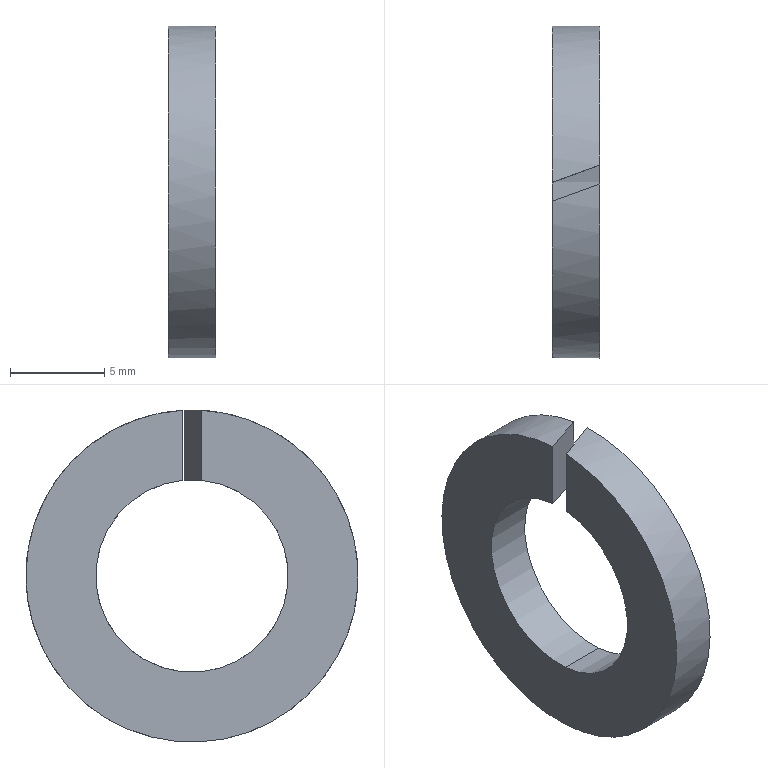Part | STEP file | KS B 1324 - No. 2 - 10 | 1 solid | 8 faces | box 2.5 x 17.6 x 17.6 mm | volume 394.643 mm3 | cylinder 4 | plane 4 | commonest cylinder face diameters 10.2 x2 17.6 x2
STEP:
#1=CARTESIAN_POINT('',(0.,0.,0.));
#2=DIRECTION('',(0.,0.,1.));
#3=DIRECTION('',(1.,0.,0.));
#4=AXIS2_PLACEMENT_3D('',#1,#2,#3);
#5=CARTESIAN_POINT('',(2.5,1.41,4.901));
#6=VERTEX_POINT('',#5);
#7=CARTESIAN_POINT('',(0.,0.5,5.075));
#8=VERTEX_POINT('',#7);
#9=CARTESIAN_POINT('',(2.5,1.41,4.901));
#10=CARTESIAN_POINT('',(1.682,1.112,4.987));
#11=CARTESIAN_POINT('',(0.8467,0.8082,5.045));
#12=CARTESIAN_POINT('',(0.,0.5,5.075));
#13=(BOUNDED_CURVE()B_SPLINE_CURVE(3,(#9,#10,#11,#12),.UNSPECIFIED.,.F.,.F.)B_SPLINE_CURVE_WITH_KNOTS((4,4),(4.432,4.614),.PIECEWISE_BEZIER_KNOTS.)CURVE()GEOMETRIC_REPRESENTATION_ITEM()RATIONAL_B_SPLINE_CURVE((1.,0.9972,0.9972,1.))REPRESENTATION_ITEM(''));
#14=CARTESIAN_POINT('',(0.,0.,0.));
#15=DIRECTION('',(1.,0.,0.));
#16=DIRECTION('',(0.,-0.08921,-0.996));
#17=AXIS2_PLACEMENT_3D('',#14,#15,#16);
#18=CYLINDRICAL_SURFACE('',#17,5.1);
#19=CARTESIAN_POINT('',(2.951,2.5));
#20=CARTESIAN_POINT('',(2.954,2.463));
#21=CARTESIAN_POINT('',(2.959,2.389));
#22=CARTESIAN_POINT('',(2.967,2.277));
#23=CARTESIAN_POINT('',(2.976,2.165));
#24=CARTESIAN_POINT('',(2.984,2.053));
#25=CARTESIAN_POINT('',(2.992,1.94));
#26=CARTESIAN_POINT('',(3.,1.828));
#27=CARTESIAN_POINT('',(3.009,1.715));
#28=CARTESIAN_POINT('',(3.017,1.602));
#29=CARTESIAN_POINT('',(3.025,1.488));
#30=CARTESIAN_POINT('',(3.033,1.375));
#31=CARTESIAN_POINT('',(3.042,1.261));
#32=CARTESIAN_POINT('',(3.05,1.147));
#33=CARTESIAN_POINT('',(3.058,1.033));
#34=CARTESIAN_POINT('',(3.067,0.9185));
#35=CARTESIAN_POINT('',(3.075,0.8041));
#36=CARTESIAN_POINT('',(3.083,0.6895));
#37=CARTESIAN_POINT('',(3.091,0.5749));
#38=CARTESIAN_POINT('',(3.1,0.4601));
#39=CARTESIAN_POINT('',(3.108,0.3452));
#40=CARTESIAN_POINT('',(3.116,0.2302));
#41=CARTESIAN_POINT('',(3.124,0.1151));
#42=CARTESIAN_POINT('',(3.13,0.03838));
#43=CARTESIAN_POINT('',(3.133,0.));
#44=B_SPLINE_CURVE_WITH_KNOTS('',3,(#19,#20,#21,#22,#23,#24,#25,#26,#27,#28,#29,#30,#31,#32,#33,#34,#35,#36,#37,#38,#39,#40,#41,#42,#43),.UNSPECIFIED.,.F.,.F.,(4,1,1,1,1,1,1,1,1,1,1,1,1,1,1,1,1,1,1,1,1,1,4),(4.432,4.441,4.449,4.457,4.465,4.474,4.482,4.49,4.498,4.507,4.515,4.523,4.532,4.54,4.548,4.556,4.565,4.573,4.581,4.589,4.598,4.606,4.614),.QUASI_UNIFORM_KNOTS.);
#45=(GEOMETRIC_REPRESENTATION_CONTEXT(2)PARAMETRIC_REPRESENTATION_CONTEXT()REPRESENTATION_CONTEXT('',''));
#46=DEFINITIONAL_REPRESENTATION('',(#44),#45);
#47=PCURVE('',#18,#46);
#48=CARTESIAN_POINT('',(0.,0.5,0.));
#49=DIRECTION('',(-0.342,0.9397,0.));
#50=DIRECTION('',(0.,0.,1.));
#51=AXIS2_PLACEMENT_3D('',#48,#49,#50);
#52=PLANE('',#51);
#53=CARTESIAN_POINT('',(4.901,2.66));
#54=CARTESIAN_POINT('',(4.987,1.79));
#55=CARTESIAN_POINT('',(5.045,0.9011));
#56=CARTESIAN_POINT('',(5.075,0.));
#57=(BOUNDED_CURVE()B_SPLINE_CURVE(3,(#53,#54,#55,#56),.UNSPECIFIED.,.F.,.F.)B_SPLINE_CURVE_WITH_KNOTS((4,4),(4.432,4.614),.PIECEWISE_BEZIER_KNOTS.)CURVE()GEOMETRIC_REPRESENTATION_ITEM()RATIONAL_B_SPLINE_CURVE((1.,0.9972,0.9972,1.))REPRESENTATION_ITEM(''));
#58=(GEOMETRIC_REPRESENTATION_CONTEXT(2)PARAMETRIC_REPRESENTATION_CONTEXT()REPRESENTATION_CONTEXT('',''));
#59=DEFINITIONAL_REPRESENTATION('',(#57),#58);
#60=PCURVE('',#52,#59);
#61=SURFACE_CURVE('',#13,(#47,#60),.PCURVE_S1.);
#62=EDGE_CURVE('',#6,#8,#61,.T.);
#63=ORIENTED_EDGE('',*,*,#62,.F.);
#64=CARTESIAN_POINT('',(2.5,-0.455,-5.08));
#65=VERTEX_POINT('',#64);
#66=CARTESIAN_POINT('',(2.5,0.,0.));
#67=DIRECTION('',(-1.,0.,0.));
#68=DIRECTION('',(0.,-1.,0.));
#69=AXIS2_PLACEMENT_3D('',#66,#67,#68);
#70=CIRCLE('',#69,5.1);
#71=CARTESIAN_POINT('',(4.802,2.5));
#72=DIRECTION('',(-1.,0.));
#73=VECTOR('',#72,1.);
#74=LINE('',#71,#73);
#75=(GEOMETRIC_REPRESENTATION_CONTEXT(2)PARAMETRIC_REPRESENTATION_CONTEXT()REPRESENTATION_CONTEXT('',''));
#76=DEFINITIONAL_REPRESENTATION('',(#74),#75);
#77=PCURVE('',#18,#76);
#78=CARTESIAN_POINT('',(2.5,0.,0.));
#79=DIRECTION('',(-1.,0.,0.));
#80=DIRECTION('',(0.,0.,1.));
#81=AXIS2_PLACEMENT_3D('',#78,#79,#80);
#82=PLANE('',#81);
#83=CARTESIAN_POINT('',(0.,0.));
#84=DIRECTION('',(0.,-1.));
#85=AXIS2_PLACEMENT_2D('',#83,#84);
#86=CIRCLE('',#85,5.1);
#87=(GEOMETRIC_REPRESENTATION_CONTEXT(2)PARAMETRIC_REPRESENTATION_CONTEXT()REPRESENTATION_CONTEXT('',''));
#88=DEFINITIONAL_REPRESENTATION('',(#86),#87);
#89=PCURVE('',#82,#88);
#90=SURFACE_CURVE('',#70,(#77,#89),.PCURVE_S1.);
#91=EDGE_CURVE('',#6,#65,#90,.T.);
#92=ORIENTED_EDGE('',*,*,#91,.T.);
#93=CARTESIAN_POINT('',(0.,-0.455,-5.08));
#94=VERTEX_POINT('',#93);
#95=CARTESIAN_POINT('',(0.,-0.455,-5.08));
#96=DIRECTION('',(1.,0.,0.));
#97=VECTOR('',#96,1.);
#98=LINE('',#95,#97);
#99=CARTESIAN_POINT('',(0.,0.));
#100=DIRECTION('',(0.,1.));
#101=VECTOR('',#100,1.);
#102=LINE('',#99,#101);
#103=(GEOMETRIC_REPRESENTATION_CONTEXT(2)PARAMETRIC_REPRESENTATION_CONTEXT()REPRESENTATION_CONTEXT('',''));
#104=DEFINITIONAL_REPRESENTATION('',(#102),#103);
#105=PCURVE('',#18,#104);
#106=CARTESIAN_POINT('',(0.,0.,0.));
#107=DIRECTION('',(1.,0.,0.));
#108=DIRECTION('',(0.,-0.08921,-0.996));
#109=AXIS2_PLACEMENT_3D('',#106,#107,#108);
#110=CYLINDRICAL_SURFACE('',#109,5.1);
#111=CARTESIAN_POINT('',(6.283,0.));
#112=DIRECTION('',(0.,1.));
#113=VECTOR('',#112,1.);
#114=LINE('',#111,#113);
#115=(GEOMETRIC_REPRESENTATION_CONTEXT(2)PARAMETRIC_REPRESENTATION_CONTEXT()REPRESENTATION_CONTEXT('',''));
#116=DEFINITIONAL_REPRESENTATION('',(#114),#115);
#117=PCURVE('',#110,#116);
#118=SURFACE_CURVE('',#98,(#105,#117),.PCURVE_S1.);
#119=EDGE_CURVE('',#94,#65,#118,.T.);
#120=ORIENTED_EDGE('',*,*,#119,.F.);
#121=CARTESIAN_POINT('',(0.,0.,0.));
#122=DIRECTION('',(1.,0.,0.));
#123=DIRECTION('',(0.,-1.,0.));
#124=AXIS2_PLACEMENT_3D('',#121,#122,#123);
#125=CIRCLE('',#124,5.1);
#126=CARTESIAN_POINT('',(-1.481,0.));
#127=DIRECTION('',(1.,0.));
#128=VECTOR('',#127,1.);
#129=LINE('',#126,#128);
#130=(GEOMETRIC_REPRESENTATION_CONTEXT(2)PARAMETRIC_REPRESENTATION_CONTEXT()REPRESENTATION_CONTEXT('',''));
#131=DEFINITIONAL_REPRESENTATION('',(#129),#130);
#132=PCURVE('',#18,#131);
#133=CARTESIAN_POINT('',(0.,0.,0.));
#134=DIRECTION('',(-1.,0.,0.));
#135=DIRECTION('',(0.,0.,1.));
#136=AXIS2_PLACEMENT_3D('',#133,#134,#135);
#137=PLANE('',#136);
#138=CARTESIAN_POINT('',(0.,-5.1));
#139=CARTESIAN_POINT('',(-8.833,-5.1));
#140=CARTESIAN_POINT('',(-4.417,2.55));
#141=CARTESIAN_POINT('',(0.,10.2));
#142=CARTESIAN_POINT('',(4.417,2.55));
#143=CARTESIAN_POINT('',(8.833,-5.1));
#144=CARTESIAN_POINT('',(0.,-5.1));
#145=(BOUNDED_CURVE()B_SPLINE_CURVE(2,(#138,#139,#140,#141,#142,#143,#144),.UNSPECIFIED.,.T.,.F.)B_SPLINE_CURVE_WITH_KNOTS((1,2,2,2,2,1),(-2.094,0.,2.094,4.189,6.283,8.378),.UNSPECIFIED.)CURVE()GEOMETRIC_REPRESENTATION_ITEM()RATIONAL_B_SPLINE_CURVE((1.,0.5,1.,0.5,1.,0.5,1.))REPRESENTATION_ITEM(''));
#146=(GEOMETRIC_REPRESENTATION_CONTEXT(2)PARAMETRIC_REPRESENTATION_CONTEXT()REPRESENTATION_CONTEXT('',''));
#147=DEFINITIONAL_REPRESENTATION('',(#145),#146);
#148=PCURVE('',#137,#147);
#149=SURFACE_CURVE('',#125,(#132,#148),.PCURVE_S1.);
#150=EDGE_CURVE('',#94,#8,#149,.T.);
#151=ORIENTED_EDGE('',*,*,#150,.T.);
#152=EDGE_LOOP('',(#63,#92,#120,#151));
#153=FACE_BOUND('',#152,.F.);
#154=ADVANCED_FACE('',(#153),#18,.F.);
#155=CARTESIAN_POINT('',(0.,-0.455,-8.788));
#156=VERTEX_POINT('',#155);
#157=CARTESIAN_POINT('',(0.,-0.5,8.786));
#158=VERTEX_POINT('',#157);
#159=CARTESIAN_POINT('',(0.,0.,0.));
#160=DIRECTION('',(-1.,0.,0.));
#161=DIRECTION('',(0.,-1.,0.));
#162=AXIS2_PLACEMENT_3D('',#159,#160,#161);
#163=CIRCLE('',#162,8.8);
#164=CARTESIAN_POINT('',(0.,0.,0.));
#165=DIRECTION('',(1.,0.,0.));
#166=DIRECTION('',(0.,-0.0517,-0.9987));
#167=AXIS2_PLACEMENT_3D('',#164,#165,#166);
#168=CYLINDRICAL_SURFACE('',#167,8.8);
#169=CARTESIAN_POINT('',(11.047,0.));
#170=DIRECTION('',(-1.,0.));
#171=VECTOR('',#170,1.);
#172=LINE('',#169,#171);
#173=(GEOMETRIC_REPRESENTATION_CONTEXT(2)PARAMETRIC_REPRESENTATION_CONTEXT()REPRESENTATION_CONTEXT('',''));
#174=DEFINITIONAL_REPRESENTATION('',(#172),#173);
#175=PCURVE('',#168,#174);
#176=CARTESIAN_POINT('',(0.,0.));
#177=DIRECTION('',(0.,-1.));
#178=AXIS2_PLACEMENT_2D('',#176,#177);
#179=CIRCLE('',#178,8.8);
#180=(GEOMETRIC_REPRESENTATION_CONTEXT(2)PARAMETRIC_REPRESENTATION_CONTEXT()REPRESENTATION_CONTEXT('',''));
#181=DEFINITIONAL_REPRESENTATION('',(#179),#180);
#182=PCURVE('',#137,#181);
#183=SURFACE_CURVE('',#163,(#175,#182),.PCURVE_S1.);
#184=EDGE_CURVE('',#156,#158,#183,.T.);
#185=ORIENTED_EDGE('',*,*,#184,.F.);
#186=CARTESIAN_POINT('',(2.5,-0.455,-8.788));
#187=VERTEX_POINT('',#186);
#188=CARTESIAN_POINT('',(0.,-0.455,-8.788));
#189=DIRECTION('',(1.,0.,0.));
#190=VECTOR('',#189,1.);
#191=LINE('',#188,#190);
#192=CARTESIAN_POINT('',(6.283,0.));
#193=DIRECTION('',(0.,1.));
#194=VECTOR('',#193,1.);
#195=LINE('',#192,#194);
#196=(GEOMETRIC_REPRESENTATION_CONTEXT(2)PARAMETRIC_REPRESENTATION_CONTEXT()REPRESENTATION_CONTEXT('',''));
#197=DEFINITIONAL_REPRESENTATION('',(#195),#196);
#198=PCURVE('',#168,#197);
#199=CARTESIAN_POINT('',(0.,0.,0.));
#200=DIRECTION('',(1.,0.,0.));
#201=DIRECTION('',(0.,-0.0517,-0.9987));
#202=AXIS2_PLACEMENT_3D('',#199,#200,#201);
#203=CYLINDRICAL_SURFACE('',#202,8.8);
#204=CARTESIAN_POINT('',(0.,0.));
#205=DIRECTION('',(0.,1.));
#206=VECTOR('',#205,1.);
#207=LINE('',#204,#206);
#208=(GEOMETRIC_REPRESENTATION_CONTEXT(2)PARAMETRIC_REPRESENTATION_CONTEXT()REPRESENTATION_CONTEXT('',''));
#209=DEFINITIONAL_REPRESENTATION('',(#207),#208);
#210=PCURVE('',#203,#209);
#211=SURFACE_CURVE('',#191,(#198,#210),.PCURVE_S1.);
#212=EDGE_CURVE('',#156,#187,#211,.T.);
#213=ORIENTED_EDGE('',*,*,#212,.T.);
#214=CARTESIAN_POINT('',(2.5,0.4099,8.79));
#215=VERTEX_POINT('',#214);
#216=CARTESIAN_POINT('',(2.5,0.,0.));
#217=DIRECTION('',(-1.,0.,0.));
#218=DIRECTION('',(0.,-1.,0.));
#219=AXIS2_PLACEMENT_3D('',#216,#217,#218);
#220=CIRCLE('',#219,8.8);
#221=CARTESIAN_POINT('',(11.047,2.5));
#222=DIRECTION('',(-1.,0.));
#223=VECTOR('',#222,1.);
#224=LINE('',#221,#223);
#225=(GEOMETRIC_REPRESENTATION_CONTEXT(2)PARAMETRIC_REPRESENTATION_CONTEXT()REPRESENTATION_CONTEXT('',''));
#226=DEFINITIONAL_REPRESENTATION('',(#224),#225);
#227=PCURVE('',#168,#226);
#228=CARTESIAN_POINT('',(0.,0.));
#229=DIRECTION('',(0.,-1.));
#230=AXIS2_PLACEMENT_2D('',#228,#229);
#231=CIRCLE('',#230,8.8);
#232=(GEOMETRIC_REPRESENTATION_CONTEXT(2)PARAMETRIC_REPRESENTATION_CONTEXT()REPRESENTATION_CONTEXT('',''));
#233=DEFINITIONAL_REPRESENTATION('',(#231),#232);
#234=PCURVE('',#82,#233);
#235=SURFACE_CURVE('',#220,(#227,#234),.PCURVE_S1.);
#236=EDGE_CURVE('',#187,#215,#235,.T.);
#237=ORIENTED_EDGE('',*,*,#236,.T.);
#238=CARTESIAN_POINT('',(2.5,0.4099,8.79));
#239=CARTESIAN_POINT('',(1.667,0.1067,8.805));
#240=CARTESIAN_POINT('',(0.8327,-0.1969,8.803));
#241=CARTESIAN_POINT('',(0.,-0.5,8.786));
#242=(BOUNDED_CURVE()B_SPLINE_CURVE(3,(#238,#239,#240,#241),.UNSPECIFIED.,.F.,.F.)B_SPLINE_CURVE_WITH_KNOTS((4,4),(4.666,4.769),.PIECEWISE_BEZIER_KNOTS.)CURVE()GEOMETRIC_REPRESENTATION_ITEM()RATIONAL_B_SPLINE_CURVE((1.,0.9991,0.9991,1.))REPRESENTATION_ITEM(''));
#243=CARTESIAN_POINT('',(3.147,2.5));
#244=CARTESIAN_POINT('',(3.148,2.462));
#245=CARTESIAN_POINT('',(3.151,2.386));
#246=CARTESIAN_POINT('',(3.156,2.273));
#247=CARTESIAN_POINT('',(3.161,2.159));
#248=CARTESIAN_POINT('',(3.166,2.046));
#249=CARTESIAN_POINT('',(3.17,1.932));
#250=CARTESIAN_POINT('',(3.175,1.818));
#251=CARTESIAN_POINT('',(3.18,1.705));
#252=CARTESIAN_POINT('',(3.184,1.591));
#253=CARTESIAN_POINT('',(3.189,1.477));
#254=CARTESIAN_POINT('',(3.194,1.364));
#255=CARTESIAN_POINT('',(3.198,1.25));
#256=CARTESIAN_POINT('',(3.203,1.136));
#257=CARTESIAN_POINT('',(3.208,1.022));
#258=CARTESIAN_POINT('',(3.213,0.9087));
#259=CARTESIAN_POINT('',(3.217,0.795));
#260=CARTESIAN_POINT('',(3.222,0.6814));
#261=CARTESIAN_POINT('',(3.227,0.5677));
#262=CARTESIAN_POINT('',(3.231,0.4541));
#263=CARTESIAN_POINT('',(3.236,0.3405));
#264=CARTESIAN_POINT('',(3.241,0.227));
#265=CARTESIAN_POINT('',(3.245,0.1135));
#266=CARTESIAN_POINT('',(3.249,0.03782));
#267=CARTESIAN_POINT('',(3.25,0.));
#268=B_SPLINE_CURVE_WITH_KNOTS('',3,(#243,#244,#245,#246,#247,#248,#249,#250,#251,#252,#253,#254,#255,#256,#257,#258,#259,#260,#261,#262,#263,#264,#265,#266,#267),.UNSPECIFIED.,.F.,.F.,(4,1,1,1,1,1,1,1,1,1,1,1,1,1,1,1,1,1,1,1,1,1,4),(4.666,4.67,4.675,4.68,4.685,4.689,4.694,4.699,4.703,4.708,4.713,4.718,4.722,4.727,4.732,4.736,4.741,4.746,4.75,4.755,4.76,4.765,4.769),.QUASI_UNIFORM_KNOTS.);
#269=(GEOMETRIC_REPRESENTATION_CONTEXT(2)PARAMETRIC_REPRESENTATION_CONTEXT()REPRESENTATION_CONTEXT('',''));
#270=DEFINITIONAL_REPRESENTATION('',(#268),#269);
#271=PCURVE('',#168,#270);
#272=CARTESIAN_POINT('',(2.5,0.4099,0.));
#273=DIRECTION('',(0.342,-0.9397,0.));
#274=DIRECTION('',(0.,0.,-1.));
#275=AXIS2_PLACEMENT_3D('',#272,#273,#274);
#276=PLANE('',#275);
#277=CARTESIAN_POINT('',(-8.79,0.));
#278=CARTESIAN_POINT('',(-8.805,-0.8867));
#279=CARTESIAN_POINT('',(-8.803,-1.774));
#280=CARTESIAN_POINT('',(-8.786,-2.66));
#281=(BOUNDED_CURVE()B_SPLINE_CURVE(3,(#277,#278,#279,#280),.UNSPECIFIED.,.F.,.F.)B_SPLINE_CURVE_WITH_KNOTS((4,4),(4.666,4.769),.PIECEWISE_BEZIER_KNOTS.)CURVE()GEOMETRIC_REPRESENTATION_ITEM()RATIONAL_B_SPLINE_CURVE((1.,0.9991,0.9991,1.))REPRESENTATION_ITEM(''));
#282=(GEOMETRIC_REPRESENTATION_CONTEXT(2)PARAMETRIC_REPRESENTATION_CONTEXT()REPRESENTATION_CONTEXT('',''));
#283=DEFINITIONAL_REPRESENTATION('',(#281),#282);
#284=PCURVE('',#276,#283);
#285=SURFACE_CURVE('',#242,(#271,#284),.PCURVE_S1.);
#286=EDGE_CURVE('',#215,#158,#285,.T.);
#287=ORIENTED_EDGE('',*,*,#286,.T.);
#288=EDGE_LOOP('',(#185,#213,#237,#287));
#289=FACE_BOUND('',#288,.T.);
#290=ADVANCED_FACE('',(#289),#168,.T.);
#291=CARTESIAN_POINT('',(0.,-0.5,5.075));
#292=VERTEX_POINT('',#291);
#293=CARTESIAN_POINT('',(0.,-0.5,0.));
#294=DIRECTION('',(0.,0.,-1.));
#295=VECTOR('',#294,1.);
#296=LINE('',#293,#295);
#297=CARTESIAN_POINT('',(0.,-0.5));
#298=DIRECTION('',(-1.,0.));
#299=VECTOR('',#298,1.);
#300=LINE('',#297,#299);
#301=(GEOMETRIC_REPRESENTATION_CONTEXT(2)PARAMETRIC_REPRESENTATION_CONTEXT()REPRESENTATION_CONTEXT('',''));
#302=DEFINITIONAL_REPRESENTATION('',(#300),#301);
#303=PCURVE('',#137,#302);
#304=CARTESIAN_POINT('',(0.,-2.66));
#305=DIRECTION('',(1.,0.));
#306=VECTOR('',#305,1.);
#307=LINE('',#304,#306);
#308=(GEOMETRIC_REPRESENTATION_CONTEXT(2)PARAMETRIC_REPRESENTATION_CONTEXT()REPRESENTATION_CONTEXT('',''));
#309=DEFINITIONAL_REPRESENTATION('',(#307),#308);
#310=PCURVE('',#276,#309);
#311=SURFACE_CURVE('',#296,(#303,#310),.PCURVE_S1.);
#312=EDGE_CURVE('',#158,#292,#311,.T.);
#313=ORIENTED_EDGE('',*,*,#312,.T.);
#314=CARTESIAN_POINT('',(0.,0.,0.));
#315=DIRECTION('',(1.,0.,0.));
#316=DIRECTION('',(0.,-1.,0.));
#317=AXIS2_PLACEMENT_3D('',#314,#315,#316);
#318=CIRCLE('',#317,5.1);
#319=CARTESIAN_POINT('',(0.,-5.1));
#320=CARTESIAN_POINT('',(-8.833,-5.1));
#321=CARTESIAN_POINT('',(-4.417,2.55));
#322=CARTESIAN_POINT('',(0.,10.2));
#323=CARTESIAN_POINT('',(4.417,2.55));
#324=CARTESIAN_POINT('',(8.833,-5.1));
#325=CARTESIAN_POINT('',(0.,-5.1));
#326=(BOUNDED_CURVE()B_SPLINE_CURVE(2,(#319,#320,#321,#322,#323,#324,#325),.UNSPECIFIED.,.T.,.F.)B_SPLINE_CURVE_WITH_KNOTS((1,2,2,2,2,1),(-2.094,0.,2.094,4.189,6.283,8.378),.UNSPECIFIED.)CURVE()GEOMETRIC_REPRESENTATION_ITEM()RATIONAL_B_SPLINE_CURVE((1.,0.5,1.,0.5,1.,0.5,1.))REPRESENTATION_ITEM(''));
#327=(GEOMETRIC_REPRESENTATION_CONTEXT(2)PARAMETRIC_REPRESENTATION_CONTEXT()REPRESENTATION_CONTEXT('',''));
#328=DEFINITIONAL_REPRESENTATION('',(#326),#327);
#329=PCURVE('',#137,#328);
#330=CARTESIAN_POINT('',(-1.481,0.));
#331=DIRECTION('',(1.,0.));
#332=VECTOR('',#331,1.);
#333=LINE('',#330,#332);
#334=(GEOMETRIC_REPRESENTATION_CONTEXT(2)PARAMETRIC_REPRESENTATION_CONTEXT()REPRESENTATION_CONTEXT('',''));
#335=DEFINITIONAL_REPRESENTATION('',(#333),#334);
#336=PCURVE('',#110,#335);
#337=SURFACE_CURVE('',#318,(#329,#336),.PCURVE_S1.);
#338=EDGE_CURVE('',#292,#94,#337,.T.);
#339=ORIENTED_EDGE('',*,*,#338,.T.);
#340=ORIENTED_EDGE('',*,*,#150,.T.);
#341=CARTESIAN_POINT('',(0.,0.5,8.786));
#342=VERTEX_POINT('',#341);
#343=CARTESIAN_POINT('',(0.,0.5,0.));
#344=DIRECTION('',(0.,0.,1.));
#345=VECTOR('',#344,1.);
#346=LINE('',#343,#345);
#347=CARTESIAN_POINT('',(0.,0.5));
#348=DIRECTION('',(1.,0.));
#349=VECTOR('',#348,1.);
#350=LINE('',#347,#349);
#351=(GEOMETRIC_REPRESENTATION_CONTEXT(2)PARAMETRIC_REPRESENTATION_CONTEXT()REPRESENTATION_CONTEXT('',''));
#352=DEFINITIONAL_REPRESENTATION('',(#350),#351);
#353=PCURVE('',#137,#352);
#354=CARTESIAN_POINT('',(0.,0.));
#355=DIRECTION('',(1.,0.));
#356=VECTOR('',#355,1.);
#357=LINE('',#354,#356);
#358=(GEOMETRIC_REPRESENTATION_CONTEXT(2)PARAMETRIC_REPRESENTATION_CONTEXT()REPRESENTATION_CONTEXT('',''));
#359=DEFINITIONAL_REPRESENTATION('',(#357),#358);
#360=PCURVE('',#52,#359);
#361=SURFACE_CURVE('',#346,(#353,#360),.PCURVE_S1.);
#362=EDGE_CURVE('',#8,#342,#361,.T.);
#363=ORIENTED_EDGE('',*,*,#362,.T.);
#364=CARTESIAN_POINT('',(0.,0.,0.));
#365=DIRECTION('',(-1.,0.,0.));
#366=DIRECTION('',(0.,-1.,0.));
#367=AXIS2_PLACEMENT_3D('',#364,#365,#366);
#368=CIRCLE('',#367,8.8);
#369=CARTESIAN_POINT('',(0.,0.));
#370=DIRECTION('',(0.,-1.));
#371=AXIS2_PLACEMENT_2D('',#369,#370);
#372=CIRCLE('',#371,8.8);
#373=(GEOMETRIC_REPRESENTATION_CONTEXT(2)PARAMETRIC_REPRESENTATION_CONTEXT()REPRESENTATION_CONTEXT('',''));
#374=DEFINITIONAL_REPRESENTATION('',(#372),#373);
#375=PCURVE('',#137,#374);
#376=CARTESIAN_POINT('',(4.764,0.));
#377=DIRECTION('',(-1.,0.));
#378=VECTOR('',#377,1.);
#379=LINE('',#376,#378);
#380=(GEOMETRIC_REPRESENTATION_CONTEXT(2)PARAMETRIC_REPRESENTATION_CONTEXT()REPRESENTATION_CONTEXT('',''));
#381=DEFINITIONAL_REPRESENTATION('',(#379),#380);
#382=PCURVE('',#203,#381);
#383=SURFACE_CURVE('',#368,(#375,#382),.PCURVE_S1.);
#384=EDGE_CURVE('',#342,#156,#383,.T.);
#385=ORIENTED_EDGE('',*,*,#384,.T.);
#386=ORIENTED_EDGE('',*,*,#184,.T.);
#387=EDGE_LOOP('',(#313,#339,#340,#363,#385,#386));
#388=FACE_BOUND('',#387,.T.);
#389=ADVANCED_FACE('',(#388),#137,.T.);
#390=ORIENTED_EDGE('',*,*,#212,.F.);
#391=ORIENTED_EDGE('',*,*,#384,.F.);
#392=CARTESIAN_POINT('',(2.5,1.41,8.686));
#393=VERTEX_POINT('',#392);
#394=CARTESIAN_POINT('',(0.,0.5,8.786));
#395=CARTESIAN_POINT('',(0.8377,0.8049,8.768));
#396=CARTESIAN_POINT('',(1.672,1.108,8.735));
#397=CARTESIAN_POINT('',(2.5,1.41,8.686));
#398=(BOUNDED_CURVE()B_SPLINE_CURVE(3,(#394,#395,#396,#397),.UNSPECIFIED.,.F.,.F.)B_SPLINE_CURVE_WITH_KNOTS((4,4),(1.628,1.732),.PIECEWISE_BEZIER_KNOTS.)CURVE()GEOMETRIC_REPRESENTATION_ITEM()RATIONAL_B_SPLINE_CURVE((1.,0.9991,0.9991,1.))REPRESENTATION_ITEM(''));
#399=CARTESIAN_POINT('',(3.136,0.));
#400=CARTESIAN_POINT('',(3.135,0.03804));
#401=CARTESIAN_POINT('',(3.132,0.1141));
#402=CARTESIAN_POINT('',(3.127,0.2282));
#403=CARTESIAN_POINT('',(3.122,0.3423));
#404=CARTESIAN_POINT('',(3.118,0.4563));
#405=CARTESIAN_POINT('',(3.113,0.5704));
#406=CARTESIAN_POINT('',(3.108,0.6843));
#407=CARTESIAN_POINT('',(3.103,0.7983));
#408=CARTESIAN_POINT('',(3.099,0.9122));
#409=CARTESIAN_POINT('',(3.094,1.026));
#410=CARTESIAN_POINT('',(3.089,1.14));
#411=CARTESIAN_POINT('',(3.084,1.254));
#412=CARTESIAN_POINT('',(3.08,1.367));
#413=CARTESIAN_POINT('',(3.075,1.481));
#414=CARTESIAN_POINT('',(3.07,1.594));
#415=CARTESIAN_POINT('',(3.066,1.708));
#416=CARTESIAN_POINT('',(3.061,1.821));
#417=CARTESIAN_POINT('',(3.056,1.935));
#418=CARTESIAN_POINT('',(3.051,2.048));
#419=CARTESIAN_POINT('',(3.047,2.161));
#420=CARTESIAN_POINT('',(3.042,2.274));
#421=CARTESIAN_POINT('',(3.037,2.387));
#422=CARTESIAN_POINT('',(3.034,2.462));
#423=CARTESIAN_POINT('',(3.032,2.5));
#424=B_SPLINE_CURVE_WITH_KNOTS('',3,(#399,#400,#401,#402,#403,#404,#405,#406,#407,#408,#409,#410,#411,#412,#413,#414,#415,#416,#417,#418,#419,#420,#421,#422,#423),.UNSPECIFIED.,.F.,.F.,(4,1,1,1,1,1,1,1,1,1,1,1,1,1,1,1,1,1,1,1,1,1,4),(1.628,1.632,1.637,1.642,1.647,1.651,1.656,1.661,1.665,1.67,1.675,1.68,1.684,1.689,1.694,1.699,1.703,1.708,1.713,1.718,1.722,1.727,1.732),.QUASI_UNIFORM_KNOTS.);
#425=(GEOMETRIC_REPRESENTATION_CONTEXT(2)PARAMETRIC_REPRESENTATION_CONTEXT()REPRESENTATION_CONTEXT('',''));
#426=DEFINITIONAL_REPRESENTATION('',(#424),#425);
#427=PCURVE('',#203,#426);
#428=CARTESIAN_POINT('',(8.786,0.));
#429=CARTESIAN_POINT('',(8.768,0.8915));
#430=CARTESIAN_POINT('',(8.735,1.779));
#431=CARTESIAN_POINT('',(8.686,2.66));
#432=(BOUNDED_CURVE()B_SPLINE_CURVE(3,(#428,#429,#430,#431),.UNSPECIFIED.,.F.,.F.)B_SPLINE_CURVE_WITH_KNOTS((4,4),(1.628,1.732),.PIECEWISE_BEZIER_KNOTS.)CURVE()GEOMETRIC_REPRESENTATION_ITEM()RATIONAL_B_SPLINE_CURVE((1.,0.9991,0.9991,1.))REPRESENTATION_ITEM(''));
#433=(GEOMETRIC_REPRESENTATION_CONTEXT(2)PARAMETRIC_REPRESENTATION_CONTEXT()REPRESENTATION_CONTEXT('',''));
#434=DEFINITIONAL_REPRESENTATION('',(#432),#433);
#435=PCURVE('',#52,#434);
#436=SURFACE_CURVE('',#398,(#427,#435),.PCURVE_S1.);
#437=EDGE_CURVE('',#342,#393,#436,.T.);
#438=ORIENTED_EDGE('',*,*,#437,.T.);
#439=CARTESIAN_POINT('',(2.5,0.,0.));
#440=DIRECTION('',(-1.,0.,0.));
#441=DIRECTION('',(0.,-1.,0.));
#442=AXIS2_PLACEMENT_3D('',#439,#440,#441);
#443=CIRCLE('',#442,8.8);
#444=CARTESIAN_POINT('',(4.764,2.5));
#445=DIRECTION('',(-1.,0.));
#446=VECTOR('',#445,1.);
#447=LINE('',#444,#446);
#448=(GEOMETRIC_REPRESENTATION_CONTEXT(2)PARAMETRIC_REPRESENTATION_CONTEXT()REPRESENTATION_CONTEXT('',''));
#449=DEFINITIONAL_REPRESENTATION('',(#447),#448);
#450=PCURVE('',#203,#449);
#451=CARTESIAN_POINT('',(0.,0.));
#452=DIRECTION('',(0.,-1.));
#453=AXIS2_PLACEMENT_2D('',#451,#452);
#454=CIRCLE('',#453,8.8);
#455=(GEOMETRIC_REPRESENTATION_CONTEXT(2)PARAMETRIC_REPRESENTATION_CONTEXT()REPRESENTATION_CONTEXT('',''));
#456=DEFINITIONAL_REPRESENTATION('',(#454),#455);
#457=PCURVE('',#82,#456);
#458=SURFACE_CURVE('',#443,(#450,#457),.PCURVE_S1.);
#459=EDGE_CURVE('',#393,#187,#458,.T.);
#460=ORIENTED_EDGE('',*,*,#459,.T.);
#461=EDGE_LOOP('',(#390,#391,#438,#460));
#462=FACE_BOUND('',#461,.T.);
#463=ADVANCED_FACE('',(#462),#203,.T.);
#464=CARTESIAN_POINT('',(2.5,0.4099,5.083));
#465=VERTEX_POINT('',#464);
#466=CARTESIAN_POINT('',(2.5,0.,0.));
#467=DIRECTION('',(-1.,0.,0.));
#468=DIRECTION('',(0.,-1.,0.));
#469=AXIS2_PLACEMENT_3D('',#466,#467,#468);
#470=CIRCLE('',#469,5.1);
#471=CARTESIAN_POINT('',(11.085,2.5));
#472=DIRECTION('',(-1.,0.));
#473=VECTOR('',#472,1.);
#474=LINE('',#471,#473);
#475=(GEOMETRIC_REPRESENTATION_CONTEXT(2)PARAMETRIC_REPRESENTATION_CONTEXT()REPRESENTATION_CONTEXT('',''));
#476=DEFINITIONAL_REPRESENTATION('',(#474),#475);
#477=PCURVE('',#110,#476);
#478=CARTESIAN_POINT('',(0.,0.));
#479=DIRECTION('',(0.,-1.));
#480=AXIS2_PLACEMENT_2D('',#478,#479);
#481=CIRCLE('',#480,5.1);
#482=(GEOMETRIC_REPRESENTATION_CONTEXT(2)PARAMETRIC_REPRESENTATION_CONTEXT()REPRESENTATION_CONTEXT('',''));
#483=DEFINITIONAL_REPRESENTATION('',(#481),#482);
#484=PCURVE('',#82,#483);
#485=SURFACE_CURVE('',#470,(#477,#484),.PCURVE_S1.);
#486=EDGE_CURVE('',#65,#465,#485,.T.);
#487=ORIENTED_EDGE('',*,*,#486,.T.);
#488=CARTESIAN_POINT('',(0.,-0.5,5.075));
#489=CARTESIAN_POINT('',(0.8316,-0.1973,5.105));
#490=CARTESIAN_POINT('',(1.667,0.1068,5.108));
#491=CARTESIAN_POINT('',(2.5,0.4099,5.083));
#492=(BOUNDED_CURVE()B_SPLINE_CURVE(3,(#488,#489,#490,#491),.UNSPECIFIED.,.F.,.F.)B_SPLINE_CURVE_WITH_KNOTS((4,4),(1.473,1.651),.PIECEWISE_BEZIER_KNOTS.)CURVE()GEOMETRIC_REPRESENTATION_ITEM()RATIONAL_B_SPLINE_CURVE((1.,0.9973,0.9973,1.))REPRESENTATION_ITEM(''));
#493=CARTESIAN_POINT('',(3.329,0.));
#494=CARTESIAN_POINT('',(3.326,0.0377));
#495=CARTESIAN_POINT('',(3.321,0.1131));
#496=CARTESIAN_POINT('',(3.313,0.2264));
#497=CARTESIAN_POINT('',(3.305,0.3398));
#498=CARTESIAN_POINT('',(3.297,0.4533));
#499=CARTESIAN_POINT('',(3.289,0.5669));
#500=CARTESIAN_POINT('',(3.28,0.6805));
#501=CARTESIAN_POINT('',(3.272,0.7942));
#502=CARTESIAN_POINT('',(3.264,0.908));
#503=CARTESIAN_POINT('',(3.256,1.022));
#504=CARTESIAN_POINT('',(3.248,1.136));
#505=CARTESIAN_POINT('',(3.24,1.25));
#506=CARTESIAN_POINT('',(3.232,1.363));
#507=CARTESIAN_POINT('',(3.224,1.477));
#508=CARTESIAN_POINT('',(3.215,1.591));
#509=CARTESIAN_POINT('',(3.207,1.705));
#510=CARTESIAN_POINT('',(3.199,1.819));
#511=CARTESIAN_POINT('',(3.191,1.932));
#512=CARTESIAN_POINT('',(3.183,2.046));
#513=CARTESIAN_POINT('',(3.175,2.16));
#514=CARTESIAN_POINT('',(3.167,2.273));
#515=CARTESIAN_POINT('',(3.159,2.387));
#516=CARTESIAN_POINT('',(3.153,2.462));
#517=CARTESIAN_POINT('',(3.15,2.5));
#518=B_SPLINE_CURVE_WITH_KNOTS('',3,(#493,#494,#495,#496,#497,#498,#499,#500,#501,#502,#503,#504,#505,#506,#507,#508,#509,#510,#511,#512,#513,#514,#515,#516,#517),.UNSPECIFIED.,.F.,.F.,(4,1,1,1,1,1,1,1,1,1,1,1,1,1,1,1,1,1,1,1,1,1,4),(1.473,1.481,1.489,1.497,1.505,1.513,1.521,1.529,1.538,1.546,1.554,1.562,1.57,1.578,1.586,1.594,1.603,1.611,1.619,1.627,1.635,1.643,1.651),.QUASI_UNIFORM_KNOTS.);
#519=(GEOMETRIC_REPRESENTATION_CONTEXT(2)PARAMETRIC_REPRESENTATION_CONTEXT()REPRESENTATION_CONTEXT('',''));
#520=DEFINITIONAL_REPRESENTATION('',(#518),#519);
#521=PCURVE('',#110,#520);
#522=CARTESIAN_POINT('',(-5.075,-2.66));
#523=CARTESIAN_POINT('',(-5.105,-1.776));
#524=CARTESIAN_POINT('',(-5.108,-0.8863));
#525=CARTESIAN_POINT('',(-5.083,0.));
#526=(BOUNDED_CURVE()B_SPLINE_CURVE(3,(#522,#523,#524,#525),.UNSPECIFIED.,.F.,.F.)B_SPLINE_CURVE_WITH_KNOTS((4,4),(1.473,1.651),.PIECEWISE_BEZIER_KNOTS.)CURVE()GEOMETRIC_REPRESENTATION_ITEM()RATIONAL_B_SPLINE_CURVE((1.,0.9973,0.9973,1.))REPRESENTATION_ITEM(''));
#527=(GEOMETRIC_REPRESENTATION_CONTEXT(2)PARAMETRIC_REPRESENTATION_CONTEXT()REPRESENTATION_CONTEXT('',''));
#528=DEFINITIONAL_REPRESENTATION('',(#526),#527);
#529=PCURVE('',#276,#528);
#530=SURFACE_CURVE('',#492,(#521,#529),.PCURVE_S1.);
#531=EDGE_CURVE('',#292,#465,#530,.T.);
#532=ORIENTED_EDGE('',*,*,#531,.F.);
#533=ORIENTED_EDGE('',*,*,#338,.T.);
#534=ORIENTED_EDGE('',*,*,#119,.T.);
#535=EDGE_LOOP('',(#487,#532,#533,#534));
#536=FACE_BOUND('',#535,.F.);
#537=ADVANCED_FACE('',(#536),#110,.F.);
#538=CARTESIAN_POINT('',(2.5,0.4099,0.));
#539=DIRECTION('',(0.,0.,1.));
#540=VECTOR('',#539,1.);
#541=LINE('',#538,#540);
#542=CARTESIAN_POINT('',(0.,0.4099));
#543=DIRECTION('',(1.,0.));
#544=VECTOR('',#543,1.);
#545=LINE('',#542,#544);
#546=(GEOMETRIC_REPRESENTATION_CONTEXT(2)PARAMETRIC_REPRESENTATION_CONTEXT()REPRESENTATION_CONTEXT('',''));
#547=DEFINITIONAL_REPRESENTATION('',(#545),#546);
#548=PCURVE('',#82,#547);
#549=CARTESIAN_POINT('',(0.,0.));
#550=DIRECTION('',(-1.,0.));
#551=VECTOR('',#550,1.);
#552=LINE('',#549,#551);
#553=(GEOMETRIC_REPRESENTATION_CONTEXT(2)PARAMETRIC_REPRESENTATION_CONTEXT()REPRESENTATION_CONTEXT('',''));
#554=DEFINITIONAL_REPRESENTATION('',(#552),#553);
#555=PCURVE('',#276,#554);
#556=SURFACE_CURVE('',#541,(#548,#555),.PCURVE_S1.);
#557=EDGE_CURVE('',#465,#215,#556,.T.);
#558=ORIENTED_EDGE('',*,*,#557,.T.);
#559=ORIENTED_EDGE('',*,*,#236,.F.);
#560=ORIENTED_EDGE('',*,*,#459,.F.);
#561=CARTESIAN_POINT('',(2.5,1.41,0.));
#562=DIRECTION('',(0.,0.,-1.));
#563=VECTOR('',#562,1.);
#564=LINE('',#561,#563);
#565=CARTESIAN_POINT('',(0.,1.41));
#566=DIRECTION('',(-1.,0.));
#567=VECTOR('',#566,1.);
#568=LINE('',#565,#567);
#569=(GEOMETRIC_REPRESENTATION_CONTEXT(2)PARAMETRIC_REPRESENTATION_CONTEXT()REPRESENTATION_CONTEXT('',''));
#570=DEFINITIONAL_REPRESENTATION('',(#568),#569);
#571=PCURVE('',#82,#570);
#572=CARTESIAN_POINT('',(0.,2.66));
#573=DIRECTION('',(-1.,0.));
#574=VECTOR('',#573,1.);
#575=LINE('',#572,#574);
#576=(GEOMETRIC_REPRESENTATION_CONTEXT(2)PARAMETRIC_REPRESENTATION_CONTEXT()REPRESENTATION_CONTEXT('',''));
#577=DEFINITIONAL_REPRESENTATION('',(#575),#576);
#578=PCURVE('',#52,#577);
#579=SURFACE_CURVE('',#564,(#571,#578),.PCURVE_S1.);
#580=EDGE_CURVE('',#393,#6,#579,.T.);
#581=ORIENTED_EDGE('',*,*,#580,.T.);
#582=ORIENTED_EDGE('',*,*,#91,.T.);
#583=ORIENTED_EDGE('',*,*,#486,.T.);
#584=EDGE_LOOP('',(#558,#559,#560,#581,#582,#583));
#585=FACE_BOUND('',#584,.T.);
#586=ADVANCED_FACE('',(#585),#82,.F.);
#587=ORIENTED_EDGE('',*,*,#531,.F.);
#588=ORIENTED_EDGE('',*,*,#312,.F.);
#589=ORIENTED_EDGE('',*,*,#286,.F.);
#590=ORIENTED_EDGE('',*,*,#557,.F.);
#591=EDGE_LOOP('',(#587,#588,#589,#590));
#592=FACE_BOUND('',#591,.T.);
#593=ADVANCED_FACE('',(#592),#276,.F.);
#594=ORIENTED_EDGE('',*,*,#62,.F.);
#595=ORIENTED_EDGE('',*,*,#580,.F.);
#596=ORIENTED_EDGE('',*,*,#437,.F.);
#597=ORIENTED_EDGE('',*,*,#362,.F.);
#598=EDGE_LOOP('',(#594,#595,#596,#597));
#599=FACE_BOUND('',#598,.T.);
#600=ADVANCED_FACE('',(#599),#52,.F.);
#601=CLOSED_SHELL('',(#154,#290,#389,#463,#537,#586,#593,#600));
#602=MANIFOLD_SOLID_BREP('',#601);
#603=(LENGTH_UNIT()NAMED_UNIT(*)SI_UNIT(.MILLI.,.METRE.));
#604=UNCERTAINTY_MEASURE_WITH_UNIT(LENGTH_MEASURE(0.0000001),#603,'','');
#605=(NAMED_UNIT(*)PLANE_ANGLE_UNIT()SI_UNIT($,.RADIAN.));
#606=(NAMED_UNIT(*)SI_UNIT($,.STERADIAN.)SOLID_ANGLE_UNIT());
#607=(GEOMETRIC_REPRESENTATION_CONTEXT(3)GLOBAL_UNCERTAINTY_ASSIGNED_CONTEXT((#604))GLOBAL_UNIT_ASSIGNED_CONTEXT((#603,#605,#606))REPRESENTATION_CONTEXT('',''));
#608=ADVANCED_BREP_SHAPE_REPRESENTATION('',(#4,#602),#607);